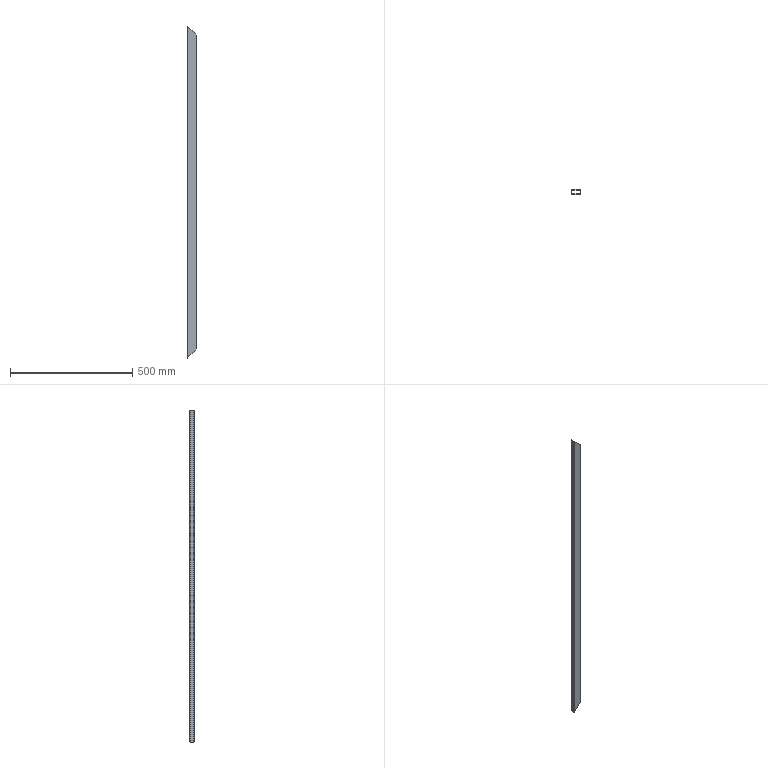Part | SolidWorks | features BaseBody 1 | 1 solid | 18 faces | box 40 x 20 x 1360 mm | volume 286615 mm3 | plane 10 | cylinder 8 | commonest cylinder face diameters 2 x4 6 x4
STEP:
#1=CARTESIAN_POINT('',(17.,-10.,643.));
#2=VERTEX_POINT('',#1);
#3=CARTESIAN_POINT('',(17.,-10.,-643.));
#4=VERTEX_POINT('',#3);
#5=CARTESIAN_POINT('',(17.,-10.,680.));
#6=DIRECTION('',(0.,0.,-1.));
#7=VECTOR('',#6,1000.);
#8=LINE('',#5,#7);
#9=EDGE_CURVE('',#2,#4,#8,.T.);
#10=ORIENTED_EDGE('',*,*,#9,.F.);
#11=CARTESIAN_POINT('',(-17.,-10.,677.));
#12=VERTEX_POINT('',#11);
#13=CARTESIAN_POINT('',(-20.,-10.,680.));
#14=DIRECTION('',(0.7071,0.,-0.7071));
#15=VECTOR('',#14,1000.);
#16=LINE('',#13,#15);
#17=EDGE_CURVE('',#12,#2,#16,.T.);
#18=ORIENTED_EDGE('',*,*,#17,.F.);
#19=CARTESIAN_POINT('',(-17.,-10.,-677.));
#20=VERTEX_POINT('',#19);
#21=CARTESIAN_POINT('',(-17.,-10.,680.));
#22=DIRECTION('',(0.,0.,-1.));
#23=VECTOR('',#22,1000.);
#24=LINE('',#21,#23);
#25=EDGE_CURVE('',#12,#20,#24,.T.);
#26=ORIENTED_EDGE('',*,*,#25,.T.);
#27=CARTESIAN_POINT('',(-20.,-10.,-680.));
#28=DIRECTION('',(-0.7071,0.,-0.7071));
#29=VECTOR('',#28,1000.);
#30=LINE('',#27,#29);
#31=EDGE_CURVE('',#4,#20,#30,.T.);
#32=ORIENTED_EDGE('',*,*,#31,.F.);
#33=EDGE_LOOP('',(#10,#18,#26,#32));
#34=FACE_OUTER_BOUND('',#33,.T.);
#35=CARTESIAN_POINT('',(-17.,-10.,680.));
#36=DIRECTION('',(0.,1.,0.));
#37=DIRECTION('',(1.,0.,0.));
#38=AXIS2_PLACEMENT_3D('',#35,#36,#37);
#39=PLANE('',#38);
#40=ADVANCED_FACE('',(#34),#39,.F.);
#41=ORIENTED_EDGE('',*,*,#25,.F.);
#42=CARTESIAN_POINT('',(-20.,-7.,680.));
#43=VERTEX_POINT('',#42);
#44=CARTESIAN_POINT('',(-17.,-10.,677.));
#45=CARTESIAN_POINT('',(-18.757,-10.,678.757));
#46=CARTESIAN_POINT('',(-20.,-8.757,680.));
#47=CARTESIAN_POINT('',(-20.,-7.,680.));
#48=(BOUNDED_CURVE()B_SPLINE_CURVE(3,(#44,#45,#46,#47),.UNSPECIFIED.,.F.,.T.)B_SPLINE_CURVE_WITH_KNOTS((4,4),(1.571,3.142),.UNSPECIFIED.)CURVE()GEOMETRIC_REPRESENTATION_ITEM()RATIONAL_B_SPLINE_CURVE((1.,0.8047,0.8047,1.))REPRESENTATION_ITEM(''));
#49=EDGE_CURVE('',#12,#43,#48,.T.);
#50=ORIENTED_EDGE('',*,*,#49,.T.);
#51=CARTESIAN_POINT('',(-20.,-7.,-680.));
#52=VERTEX_POINT('',#51);
#53=CARTESIAN_POINT('',(-20.,-7.,680.));
#54=DIRECTION('',(0.,0.,-1.));
#55=VECTOR('',#54,1000.);
#56=LINE('',#53,#55);
#57=EDGE_CURVE('',#43,#52,#56,.T.);
#58=ORIENTED_EDGE('',*,*,#57,.T.);
#59=CARTESIAN_POINT('',(-20.,-7.,-680.));
#60=CARTESIAN_POINT('',(-20.,-8.757,-680.));
#61=CARTESIAN_POINT('',(-18.757,-10.,-678.757));
#62=CARTESIAN_POINT('',(-17.,-10.,-677.));
#63=(BOUNDED_CURVE()B_SPLINE_CURVE(3,(#59,#60,#61,#62),.UNSPECIFIED.,.F.,.T.)B_SPLINE_CURVE_WITH_KNOTS((4,4),(0.,1.571),.UNSPECIFIED.)CURVE()GEOMETRIC_REPRESENTATION_ITEM()RATIONAL_B_SPLINE_CURVE((1.,0.8047,0.8047,1.))REPRESENTATION_ITEM(''));
#64=EDGE_CURVE('',#52,#20,#63,.T.);
#65=ORIENTED_EDGE('',*,*,#64,.T.);
#66=EDGE_LOOP('',(#41,#50,#58,#65));
#67=FACE_OUTER_BOUND('',#66,.T.);
#68=CARTESIAN_POINT('',(-17.,-7.,680.));
#69=DIRECTION('',(0.,0.,-1.));
#70=DIRECTION('',(-1.,0.,0.));
#71=AXIS2_PLACEMENT_3D('',#68,#69,#70);
#72=CYLINDRICAL_SURFACE('',#71,3.);
#73=ADVANCED_FACE('',(#67),#72,.T.);
#74=CARTESIAN_POINT('',(-20.,7.,-680.));
#75=VERTEX_POINT('',#74);
#76=CARTESIAN_POINT('',(-20.,7.,-680.));
#77=DIRECTION('',(0.,-1.,0.));
#78=VECTOR('',#77,1000.);
#79=LINE('',#76,#78);
#80=EDGE_CURVE('',#75,#52,#79,.T.);
#81=ORIENTED_EDGE('',*,*,#80,.T.);
#82=ORIENTED_EDGE('',*,*,#57,.F.);
#83=CARTESIAN_POINT('',(-20.,7.,680.));
#84=VERTEX_POINT('',#83);
#85=CARTESIAN_POINT('',(-20.,7.,680.));
#86=DIRECTION('',(0.,-1.,0.));
#87=VECTOR('',#86,1000.);
#88=LINE('',#85,#87);
#89=EDGE_CURVE('',#84,#43,#88,.T.);
#90=ORIENTED_EDGE('',*,*,#89,.F.);
#91=CARTESIAN_POINT('',(-20.,7.,680.));
#92=DIRECTION('',(0.,0.,-1.));
#93=VECTOR('',#92,1000.);
#94=LINE('',#91,#93);
#95=EDGE_CURVE('',#84,#75,#94,.T.);
#96=ORIENTED_EDGE('',*,*,#95,.T.);
#97=EDGE_LOOP('',(#81,#82,#90,#96));
#98=FACE_OUTER_BOUND('',#97,.T.);
#99=CARTESIAN_POINT('',(-20.,7.,680.));
#100=DIRECTION('',(1.,0.,0.));
#101=DIRECTION('',(0.,1.,0.));
#102=AXIS2_PLACEMENT_3D('',#99,#100,#101);
#103=PLANE('',#102);
#104=ADVANCED_FACE('',(#98),#103,.F.);
#105=ORIENTED_EDGE('',*,*,#95,.F.);
#106=CARTESIAN_POINT('',(-17.,10.,677.));
#107=VERTEX_POINT('',#106);
#108=CARTESIAN_POINT('',(-20.,7.,680.));
#109=CARTESIAN_POINT('',(-20.,8.757,680.));
#110=CARTESIAN_POINT('',(-18.757,10.,678.757));
#111=CARTESIAN_POINT('',(-17.,10.,677.));
#112=(BOUNDED_CURVE()B_SPLINE_CURVE(3,(#108,#109,#110,#111),.UNSPECIFIED.,.F.,.T.)B_SPLINE_CURVE_WITH_KNOTS((4,4),(3.142,4.712),.UNSPECIFIED.)CURVE()GEOMETRIC_REPRESENTATION_ITEM()RATIONAL_B_SPLINE_CURVE((1.,0.8047,0.8047,1.))REPRESENTATION_ITEM(''));
#113=EDGE_CURVE('',#84,#107,#112,.T.);
#114=ORIENTED_EDGE('',*,*,#113,.T.);
#115=CARTESIAN_POINT('',(-17.,10.,-677.));
#116=VERTEX_POINT('',#115);
#117=CARTESIAN_POINT('',(-17.,10.,680.));
#118=DIRECTION('',(0.,0.,-1.));
#119=VECTOR('',#118,1000.);
#120=LINE('',#117,#119);
#121=EDGE_CURVE('',#107,#116,#120,.T.);
#122=ORIENTED_EDGE('',*,*,#121,.T.);
#123=CARTESIAN_POINT('',(-17.,10.,-677.));
#124=CARTESIAN_POINT('',(-18.757,10.,-678.757));
#125=CARTESIAN_POINT('',(-20.,8.757,-680.));
#126=CARTESIAN_POINT('',(-20.,7.,-680.));
#127=(BOUNDED_CURVE()B_SPLINE_CURVE(3,(#123,#124,#125,#126),.UNSPECIFIED.,.F.,.F.)B_SPLINE_CURVE_WITH_KNOTS((4,4),(4.712,6.283),.UNSPECIFIED.)CURVE()GEOMETRIC_REPRESENTATION_ITEM()RATIONAL_B_SPLINE_CURVE((1.,0.8047,0.8047,1.))REPRESENTATION_ITEM(''));
#128=EDGE_CURVE('',#116,#75,#127,.T.);
#129=ORIENTED_EDGE('',*,*,#128,.T.);
#130=EDGE_LOOP('',(#105,#114,#122,#129));
#131=FACE_OUTER_BOUND('',#130,.T.);
#132=CARTESIAN_POINT('',(-17.,7.,680.));
#133=DIRECTION('',(0.,0.,-1.));
#134=DIRECTION('',(-1.,0.,0.));
#135=AXIS2_PLACEMENT_3D('',#132,#133,#134);
#136=CYLINDRICAL_SURFACE('',#135,3.);
#137=ADVANCED_FACE('',(#131),#136,.T.);
#138=ORIENTED_EDGE('',*,*,#121,.F.);
#139=CARTESIAN_POINT('',(17.,10.,643.));
#140=VERTEX_POINT('',#139);
#141=CARTESIAN_POINT('',(-20.,10.,680.));
#142=DIRECTION('',(0.7071,0.,-0.7071));
#143=VECTOR('',#142,1000.);
#144=LINE('',#141,#143);
#145=EDGE_CURVE('',#107,#140,#144,.T.);
#146=ORIENTED_EDGE('',*,*,#145,.T.);
#147=CARTESIAN_POINT('',(17.,10.,-643.));
#148=VERTEX_POINT('',#147);
#149=CARTESIAN_POINT('',(17.,10.,680.));
#150=DIRECTION('',(0.,0.,-1.));
#151=VECTOR('',#150,1000.);
#152=LINE('',#149,#151);
#153=EDGE_CURVE('',#140,#148,#152,.T.);
#154=ORIENTED_EDGE('',*,*,#153,.T.);
#155=CARTESIAN_POINT('',(-20.,10.,-680.));
#156=DIRECTION('',(-0.7071,0.,-0.7071));
#157=VECTOR('',#156,1000.);
#158=LINE('',#155,#157);
#159=EDGE_CURVE('',#148,#116,#158,.T.);
#160=ORIENTED_EDGE('',*,*,#159,.T.);
#161=EDGE_LOOP('',(#138,#146,#154,#160));
#162=FACE_OUTER_BOUND('',#161,.T.);
#163=CARTESIAN_POINT('',(-17.,10.,680.));
#164=DIRECTION('',(0.,-1.,0.));
#165=DIRECTION('',(0.,0.,-1.));
#166=AXIS2_PLACEMENT_3D('',#163,#164,#165);
#167=PLANE('',#166);
#168=ADVANCED_FACE('',(#162),#167,.F.);
#169=ORIENTED_EDGE('',*,*,#153,.F.);
#170=CARTESIAN_POINT('',(20.,7.,640.));
#171=VERTEX_POINT('',#170);
#172=CARTESIAN_POINT('',(17.,10.,643.));
#173=CARTESIAN_POINT('',(18.757,10.,641.243));
#174=CARTESIAN_POINT('',(20.,8.757,640.));
#175=CARTESIAN_POINT('',(20.,7.,640.));
#176=(BOUNDED_CURVE()B_SPLINE_CURVE(3,(#172,#173,#174,#175),.UNSPECIFIED.,.F.,.T.)B_SPLINE_CURVE_WITH_KNOTS((4,4),(4.712,6.283),.UNSPECIFIED.)CURVE()GEOMETRIC_REPRESENTATION_ITEM()RATIONAL_B_SPLINE_CURVE((1.,0.8047,0.8047,1.))REPRESENTATION_ITEM(''));
#177=EDGE_CURVE('',#140,#171,#176,.T.);
#178=ORIENTED_EDGE('',*,*,#177,.T.);
#179=CARTESIAN_POINT('',(20.,7.,-640.));
#180=VERTEX_POINT('',#179);
#181=CARTESIAN_POINT('',(20.,7.,680.));
#182=DIRECTION('',(0.,0.,-1.));
#183=VECTOR('',#182,1000.);
#184=LINE('',#181,#183);
#185=EDGE_CURVE('',#171,#180,#184,.T.);
#186=ORIENTED_EDGE('',*,*,#185,.T.);
#187=CARTESIAN_POINT('',(20.,7.,-640.));
#188=CARTESIAN_POINT('',(20.,8.757,-640.));
#189=CARTESIAN_POINT('',(18.757,10.,-641.243));
#190=CARTESIAN_POINT('',(17.,10.,-643.));
#191=(BOUNDED_CURVE()B_SPLINE_CURVE(3,(#187,#188,#189,#190),.UNSPECIFIED.,.F.,.T.)B_SPLINE_CURVE_WITH_KNOTS((4,4),(3.142,4.712),.UNSPECIFIED.)CURVE()GEOMETRIC_REPRESENTATION_ITEM()RATIONAL_B_SPLINE_CURVE((1.,0.8047,0.8047,1.))REPRESENTATION_ITEM(''));
#192=EDGE_CURVE('',#180,#148,#191,.T.);
#193=ORIENTED_EDGE('',*,*,#192,.T.);
#194=EDGE_LOOP('',(#169,#178,#186,#193));
#195=FACE_OUTER_BOUND('',#194,.T.);
#196=CARTESIAN_POINT('',(17.,7.,680.));
#197=DIRECTION('',(0.,0.,-1.));
#198=DIRECTION('',(-1.,0.,0.));
#199=AXIS2_PLACEMENT_3D('',#196,#197,#198);
#200=CYLINDRICAL_SURFACE('',#199,3.);
#201=ADVANCED_FACE('',(#195),#200,.T.);
#202=ORIENTED_EDGE('',*,*,#185,.F.);
#203=CARTESIAN_POINT('',(20.,-7.,640.));
#204=VERTEX_POINT('',#203);
#205=CARTESIAN_POINT('',(20.,10.,640.));
#206=DIRECTION('',(0.,-1.,0.));
#207=VECTOR('',#206,1000.);
#208=LINE('',#205,#207);
#209=EDGE_CURVE('',#171,#204,#208,.T.);
#210=ORIENTED_EDGE('',*,*,#209,.T.);
#211=CARTESIAN_POINT('',(20.,-7.,-640.));
#212=VERTEX_POINT('',#211);
#213=CARTESIAN_POINT('',(20.,-7.,680.));
#214=DIRECTION('',(0.,0.,-1.));
#215=VECTOR('',#214,1000.);
#216=LINE('',#213,#215);
#217=EDGE_CURVE('',#204,#212,#216,.T.);
#218=ORIENTED_EDGE('',*,*,#217,.T.);
#219=CARTESIAN_POINT('',(20.,10.,-640.));
#220=DIRECTION('',(0.,-1.,0.));
#221=VECTOR('',#220,1000.);
#222=LINE('',#219,#221);
#223=EDGE_CURVE('',#180,#212,#222,.T.);
#224=ORIENTED_EDGE('',*,*,#223,.F.);
#225=EDGE_LOOP('',(#202,#210,#218,#224));
#226=FACE_OUTER_BOUND('',#225,.T.);
#227=CARTESIAN_POINT('',(20.,7.,680.));
#228=DIRECTION('',(-1.,0.,0.));
#229=DIRECTION('',(0.,0.,1.));
#230=AXIS2_PLACEMENT_3D('',#227,#228,#229);
#231=PLANE('',#230);
#232=ADVANCED_FACE('',(#226),#231,.F.);
#233=ORIENTED_EDGE('',*,*,#217,.F.);
#234=CARTESIAN_POINT('',(20.,-7.,640.));
#235=CARTESIAN_POINT('',(20.,-8.757,640.));
#236=CARTESIAN_POINT('',(18.757,-10.,641.243));
#237=CARTESIAN_POINT('',(17.,-10.,643.));
#238=(BOUNDED_CURVE()B_SPLINE_CURVE(3,(#234,#235,#236,#237),.UNSPECIFIED.,.F.,.T.)B_SPLINE_CURVE_WITH_KNOTS((4,4),(0.,1.571),.UNSPECIFIED.)CURVE()GEOMETRIC_REPRESENTATION_ITEM()RATIONAL_B_SPLINE_CURVE((1.,0.8047,0.8047,1.))REPRESENTATION_ITEM(''));
#239=EDGE_CURVE('',#204,#2,#238,.T.);
#240=ORIENTED_EDGE('',*,*,#239,.T.);
#241=ORIENTED_EDGE('',*,*,#9,.T.);
#242=CARTESIAN_POINT('',(17.,-10.,-643.));
#243=CARTESIAN_POINT('',(18.757,-10.,-641.243));
#244=CARTESIAN_POINT('',(20.,-8.757,-640.));
#245=CARTESIAN_POINT('',(20.,-7.,-640.));
#246=(BOUNDED_CURVE()B_SPLINE_CURVE(3,(#242,#243,#244,#245),.UNSPECIFIED.,.F.,.T.)B_SPLINE_CURVE_WITH_KNOTS((4,4),(1.571,3.142),.UNSPECIFIED.)CURVE()GEOMETRIC_REPRESENTATION_ITEM()RATIONAL_B_SPLINE_CURVE((1.,0.8047,0.8047,1.))REPRESENTATION_ITEM(''));
#247=EDGE_CURVE('',#4,#212,#246,.T.);
#248=ORIENTED_EDGE('',*,*,#247,.T.);
#249=EDGE_LOOP('',(#233,#240,#241,#248));
#250=FACE_OUTER_BOUND('',#249,.T.);
#251=CARTESIAN_POINT('',(17.,-7.,680.));
#252=DIRECTION('',(0.,0.,-1.));
#253=DIRECTION('',(-1.,0.,0.));
#254=AXIS2_PLACEMENT_3D('',#251,#252,#253);
#255=CYLINDRICAL_SURFACE('',#254,3.);
#256=ADVANCED_FACE('',(#250),#255,.T.);
#257=CARTESIAN_POINT('',(17.,8.,643.));
#258=VERTEX_POINT('',#257);
#259=CARTESIAN_POINT('',(18.,7.,642.));
#260=VERTEX_POINT('',#259);
#261=CARTESIAN_POINT('',(17.,8.,643.));
#262=CARTESIAN_POINT('',(17.586,8.,642.414));
#263=CARTESIAN_POINT('',(18.,7.586,642.));
#264=CARTESIAN_POINT('',(18.,7.,642.));
#265=(BOUNDED_CURVE()B_SPLINE_CURVE(3,(#261,#262,#263,#264),.UNSPECIFIED.,.F.,.F.)B_SPLINE_CURVE_WITH_KNOTS((4,4),(4.712,6.283),.UNSPECIFIED.)CURVE()GEOMETRIC_REPRESENTATION_ITEM()RATIONAL_B_SPLINE_CURVE((1.,0.8047,0.8047,1.))REPRESENTATION_ITEM(''));
#266=EDGE_CURVE('',#258,#260,#265,.T.);
#267=ORIENTED_EDGE('',*,*,#266,.T.);
#268=CARTESIAN_POINT('',(18.,-7.,642.));
#269=VERTEX_POINT('',#268);
#270=CARTESIAN_POINT('',(18.,7.,642.));
#271=DIRECTION('',(0.,-1.,0.));
#272=VECTOR('',#271,1000.);
#273=LINE('',#270,#272);
#274=EDGE_CURVE('',#260,#269,#273,.T.);
#275=ORIENTED_EDGE('',*,*,#274,.T.);
#276=CARTESIAN_POINT('',(17.,-8.,643.));
#277=VERTEX_POINT('',#276);
#278=CARTESIAN_POINT('',(18.,-7.,642.));
#279=CARTESIAN_POINT('',(18.,-7.586,642.));
#280=CARTESIAN_POINT('',(17.586,-8.,642.414));
#281=CARTESIAN_POINT('',(17.,-8.,643.));
#282=(BOUNDED_CURVE()B_SPLINE_CURVE(3,(#278,#279,#280,#281),.UNSPECIFIED.,.F.,.T.)B_SPLINE_CURVE_WITH_KNOTS((4,4),(0.,1.571),.UNSPECIFIED.)CURVE()GEOMETRIC_REPRESENTATION_ITEM()RATIONAL_B_SPLINE_CURVE((1.,0.8047,0.8047,1.))REPRESENTATION_ITEM(''));
#283=EDGE_CURVE('',#269,#277,#282,.T.);
#284=ORIENTED_EDGE('',*,*,#283,.T.);
#285=CARTESIAN_POINT('',(-17.,-8.,677.));
#286=VERTEX_POINT('',#285);
#287=CARTESIAN_POINT('',(-18.5,-8.,678.5));
#288=DIRECTION('',(-0.7071,0.,0.7071));
#289=VECTOR('',#288,1000.);
#290=LINE('',#287,#289);
#291=EDGE_CURVE('',#277,#286,#290,.T.);
#292=ORIENTED_EDGE('',*,*,#291,.T.);
#293=CARTESIAN_POINT('',(-18.,-7.,678.));
#294=VERTEX_POINT('',#293);
#295=CARTESIAN_POINT('',(-17.,-8.,677.));
#296=CARTESIAN_POINT('',(-17.586,-8.,677.586));
#297=CARTESIAN_POINT('',(-18.,-7.586,678.));
#298=CARTESIAN_POINT('',(-18.,-7.,678.));
#299=(BOUNDED_CURVE()B_SPLINE_CURVE(3,(#295,#296,#297,#298),.UNSPECIFIED.,.F.,.T.)B_SPLINE_CURVE_WITH_KNOTS((4,4),(1.571,3.142),.UNSPECIFIED.)CURVE()GEOMETRIC_REPRESENTATION_ITEM()RATIONAL_B_SPLINE_CURVE((1.,0.8047,0.8047,1.))REPRESENTATION_ITEM(''));
#300=EDGE_CURVE('',#286,#294,#299,.T.);
#301=ORIENTED_EDGE('',*,*,#300,.T.);
#302=CARTESIAN_POINT('',(-18.,7.,678.));
#303=VERTEX_POINT('',#302);
#304=CARTESIAN_POINT('',(-18.,7.,678.));
#305=DIRECTION('',(0.,1.,0.));
#306=VECTOR('',#305,1000.);
#307=LINE('',#304,#306);
#308=EDGE_CURVE('',#294,#303,#307,.T.);
#309=ORIENTED_EDGE('',*,*,#308,.T.);
#310=CARTESIAN_POINT('',(-17.,8.,677.));
#311=VERTEX_POINT('',#310);
#312=CARTESIAN_POINT('',(-18.,7.,678.));
#313=CARTESIAN_POINT('',(-18.,7.586,678.));
#314=CARTESIAN_POINT('',(-17.586,8.,677.586));
#315=CARTESIAN_POINT('',(-17.,8.,677.));
#316=(BOUNDED_CURVE()B_SPLINE_CURVE(3,(#312,#313,#314,#315),.UNSPECIFIED.,.F.,.T.)B_SPLINE_CURVE_WITH_KNOTS((4,4),(3.142,4.712),.UNSPECIFIED.)CURVE()GEOMETRIC_REPRESENTATION_ITEM()RATIONAL_B_SPLINE_CURVE((1.,0.8047,0.8047,1.))REPRESENTATION_ITEM(''));
#317=EDGE_CURVE('',#303,#311,#316,.T.);
#318=ORIENTED_EDGE('',*,*,#317,.T.);
#319=CARTESIAN_POINT('',(-18.5,8.,678.5));
#320=DIRECTION('',(0.7071,0.,-0.7071));
#321=VECTOR('',#320,1000.);
#322=LINE('',#319,#321);
#323=EDGE_CURVE('',#311,#258,#322,.T.);
#324=ORIENTED_EDGE('',*,*,#323,.T.);
#325=EDGE_LOOP('',(#267,#275,#284,#292,#301,#309,#318,#324));
#326=FACE_BOUND('',#325,.T.);
#327=ORIENTED_EDGE('',*,*,#209,.F.);
#328=ORIENTED_EDGE('',*,*,#177,.F.);
#329=ORIENTED_EDGE('',*,*,#145,.F.);
#330=ORIENTED_EDGE('',*,*,#113,.F.);
#331=ORIENTED_EDGE('',*,*,#89,.T.);
#332=ORIENTED_EDGE('',*,*,#49,.F.);
#333=ORIENTED_EDGE('',*,*,#17,.T.);
#334=ORIENTED_EDGE('',*,*,#239,.F.);
#335=EDGE_LOOP('',(#327,#328,#329,#330,#331,#332,#333,#334));
#336=FACE_OUTER_BOUND('',#335,.T.);
#337=CARTESIAN_POINT('',(-20.,10.,680.));
#338=DIRECTION('',(-0.7071,0.,-0.7071));
#339=DIRECTION('',(-0.7071,0.,0.7071));
#340=AXIS2_PLACEMENT_3D('',#337,#338,#339);
#341=PLANE('',#340);
#342=ADVANCED_FACE('',(#326,#336),#341,.F.);
#343=CARTESIAN_POINT('',(18.,7.,-642.));
#344=VERTEX_POINT('',#343);
#345=CARTESIAN_POINT('',(17.,8.,-643.));
#346=VERTEX_POINT('',#345);
#347=CARTESIAN_POINT('',(18.,7.,-642.));
#348=CARTESIAN_POINT('',(18.,7.586,-642.));
#349=CARTESIAN_POINT('',(17.586,8.,-642.414));
#350=CARTESIAN_POINT('',(17.,8.,-643.));
#351=(BOUNDED_CURVE()B_SPLINE_CURVE(3,(#347,#348,#349,#350),.UNSPECIFIED.,.F.,.T.)B_SPLINE_CURVE_WITH_KNOTS((4,4),(3.142,4.712),.UNSPECIFIED.)CURVE()GEOMETRIC_REPRESENTATION_ITEM()RATIONAL_B_SPLINE_CURVE((1.,0.8047,0.8047,1.))REPRESENTATION_ITEM(''));
#352=EDGE_CURVE('',#344,#346,#351,.T.);
#353=ORIENTED_EDGE('',*,*,#352,.T.);
#354=CARTESIAN_POINT('',(-17.,8.,-677.));
#355=VERTEX_POINT('',#354);
#356=CARTESIAN_POINT('',(661.5,8.,1.5));
#357=DIRECTION('',(-0.7071,0.,-0.7071));
#358=VECTOR('',#357,1000.);
#359=LINE('',#356,#358);
#360=EDGE_CURVE('',#346,#355,#359,.T.);
#361=ORIENTED_EDGE('',*,*,#360,.T.);
#362=CARTESIAN_POINT('',(-18.,7.,-678.));
#363=VERTEX_POINT('',#362);
#364=CARTESIAN_POINT('',(-17.,8.,-677.));
#365=CARTESIAN_POINT('',(-17.586,8.,-677.586));
#366=CARTESIAN_POINT('',(-18.,7.586,-678.));
#367=CARTESIAN_POINT('',(-18.,7.,-678.));
#368=(BOUNDED_CURVE()B_SPLINE_CURVE(3,(#364,#365,#366,#367),.UNSPECIFIED.,.F.,.T.)B_SPLINE_CURVE_WITH_KNOTS((4,4),(4.712,6.283),.UNSPECIFIED.)CURVE()GEOMETRIC_REPRESENTATION_ITEM()RATIONAL_B_SPLINE_CURVE((1.,0.8047,0.8047,1.))REPRESENTATION_ITEM(''));
#369=EDGE_CURVE('',#355,#363,#368,.T.);
#370=ORIENTED_EDGE('',*,*,#369,.T.);
#371=CARTESIAN_POINT('',(-18.,-7.,-678.));
#372=VERTEX_POINT('',#371);
#373=CARTESIAN_POINT('',(-18.,7.,-678.));
#374=DIRECTION('',(0.,-1.,0.));
#375=VECTOR('',#374,1000.);
#376=LINE('',#373,#375);
#377=EDGE_CURVE('',#363,#372,#376,.T.);
#378=ORIENTED_EDGE('',*,*,#377,.T.);
#379=CARTESIAN_POINT('',(-17.,-8.,-677.));
#380=VERTEX_POINT('',#379);
#381=CARTESIAN_POINT('',(-18.,-7.,-678.));
#382=CARTESIAN_POINT('',(-18.,-7.586,-678.));
#383=CARTESIAN_POINT('',(-17.586,-8.,-677.586));
#384=CARTESIAN_POINT('',(-17.,-8.,-677.));
#385=(BOUNDED_CURVE()B_SPLINE_CURVE(3,(#381,#382,#383,#384),.UNSPECIFIED.,.F.,.T.)B_SPLINE_CURVE_WITH_KNOTS((4,4),(0.,1.571),.UNSPECIFIED.)CURVE()GEOMETRIC_REPRESENTATION_ITEM()RATIONAL_B_SPLINE_CURVE((1.,0.8047,0.8047,1.))REPRESENTATION_ITEM(''));
#386=EDGE_CURVE('',#372,#380,#385,.T.);
#387=ORIENTED_EDGE('',*,*,#386,.T.);
#388=CARTESIAN_POINT('',(17.,-8.,-643.));
#389=VERTEX_POINT('',#388);
#390=CARTESIAN_POINT('',(661.5,-8.,1.5));
#391=DIRECTION('',(0.7071,0.,0.7071));
#392=VECTOR('',#391,1000.);
#393=LINE('',#390,#392);
#394=EDGE_CURVE('',#380,#389,#393,.T.);
#395=ORIENTED_EDGE('',*,*,#394,.T.);
#396=CARTESIAN_POINT('',(18.,-7.,-642.));
#397=VERTEX_POINT('',#396);
#398=CARTESIAN_POINT('',(17.,-8.,-643.));
#399=CARTESIAN_POINT('',(17.586,-8.,-642.414));
#400=CARTESIAN_POINT('',(18.,-7.586,-642.));
#401=CARTESIAN_POINT('',(18.,-7.,-642.));
#402=(BOUNDED_CURVE()B_SPLINE_CURVE(3,(#398,#399,#400,#401),.UNSPECIFIED.,.F.,.T.)B_SPLINE_CURVE_WITH_KNOTS((4,4),(1.571,3.142),.UNSPECIFIED.)CURVE()GEOMETRIC_REPRESENTATION_ITEM()RATIONAL_B_SPLINE_CURVE((1.,0.8047,0.8047,1.))REPRESENTATION_ITEM(''));
#403=EDGE_CURVE('',#389,#397,#402,.T.);
#404=ORIENTED_EDGE('',*,*,#403,.T.);
#405=CARTESIAN_POINT('',(18.,7.,-642.));
#406=DIRECTION('',(0.,1.,0.));
#407=VECTOR('',#406,1000.);
#408=LINE('',#405,#407);
#409=EDGE_CURVE('',#397,#344,#408,.T.);
#410=ORIENTED_EDGE('',*,*,#409,.T.);
#411=EDGE_LOOP('',(#353,#361,#370,#378,#387,#395,#404,#410));
#412=FACE_BOUND('',#411,.T.);
#413=ORIENTED_EDGE('',*,*,#31,.T.);
#414=ORIENTED_EDGE('',*,*,#64,.F.);
#415=ORIENTED_EDGE('',*,*,#80,.F.);
#416=ORIENTED_EDGE('',*,*,#128,.F.);
#417=ORIENTED_EDGE('',*,*,#159,.F.);
#418=ORIENTED_EDGE('',*,*,#192,.F.);
#419=ORIENTED_EDGE('',*,*,#223,.T.);
#420=ORIENTED_EDGE('',*,*,#247,.F.);
#421=EDGE_LOOP('',(#413,#414,#415,#416,#417,#418,#419,#420));
#422=FACE_OUTER_BOUND('',#421,.T.);
#423=CARTESIAN_POINT('',(-20.,10.,-680.));
#424=DIRECTION('',(-0.7071,0.,0.7071));
#425=DIRECTION('',(0.,1.,0.));
#426=AXIS2_PLACEMENT_3D('',#423,#424,#425);
#427=PLANE('',#426);
#428=ADVANCED_FACE('',(#412,#422),#427,.F.);
#429=ORIENTED_EDGE('',*,*,#266,.F.);
#430=CARTESIAN_POINT('',(17.,8.,680.));
#431=DIRECTION('',(0.,0.,-1.));
#432=VECTOR('',#431,1000.);
#433=LINE('',#430,#432);
#434=EDGE_CURVE('',#258,#346,#433,.T.);
#435=ORIENTED_EDGE('',*,*,#434,.T.);
#436=ORIENTED_EDGE('',*,*,#352,.F.);
#437=CARTESIAN_POINT('',(18.,7.,680.));
#438=DIRECTION('',(0.,0.,-1.));
#439=VECTOR('',#438,1000.);
#440=LINE('',#437,#439);
#441=EDGE_CURVE('',#260,#344,#440,.T.);
#442=ORIENTED_EDGE('',*,*,#441,.F.);
#443=EDGE_LOOP('',(#429,#435,#436,#442));
#444=FACE_OUTER_BOUND('',#443,.T.);
#445=CARTESIAN_POINT('',(17.,7.,680.));
#446=DIRECTION('',(0.,0.,-1.));
#447=DIRECTION('',(-1.,0.,0.));
#448=AXIS2_PLACEMENT_3D('',#445,#446,#447);
#449=CYLINDRICAL_SURFACE('',#448,1.);
#450=ADVANCED_FACE('',(#444),#449,.F.);
#451=ORIENTED_EDGE('',*,*,#323,.F.);
#452=CARTESIAN_POINT('',(-17.,8.,680.));
#453=DIRECTION('',(0.,0.,-1.));
#454=VECTOR('',#453,1000.);
#455=LINE('',#452,#454);
#456=EDGE_CURVE('',#311,#355,#455,.T.);
#457=ORIENTED_EDGE('',*,*,#456,.T.);
#458=ORIENTED_EDGE('',*,*,#360,.F.);
#459=ORIENTED_EDGE('',*,*,#434,.F.);
#460=EDGE_LOOP('',(#451,#457,#458,#459));
#461=FACE_OUTER_BOUND('',#460,.T.);
#462=CARTESIAN_POINT('',(-17.,8.,680.));
#463=DIRECTION('',(0.,-1.,0.));
#464=DIRECTION('',(0.,0.,-1.));
#465=AXIS2_PLACEMENT_3D('',#462,#463,#464);
#466=PLANE('',#465);
#467=ADVANCED_FACE('',(#461),#466,.T.);
#468=ORIENTED_EDGE('',*,*,#317,.F.);
#469=CARTESIAN_POINT('',(-18.,7.,680.));
#470=DIRECTION('',(0.,0.,-1.));
#471=VECTOR('',#470,1000.);
#472=LINE('',#469,#471);
#473=EDGE_CURVE('',#303,#363,#472,.T.);
#474=ORIENTED_EDGE('',*,*,#473,.T.);
#475=ORIENTED_EDGE('',*,*,#369,.F.);
#476=ORIENTED_EDGE('',*,*,#456,.F.);
#477=EDGE_LOOP('',(#468,#474,#475,#476));
#478=FACE_OUTER_BOUND('',#477,.T.);
#479=CARTESIAN_POINT('',(-17.,7.,680.));
#480=DIRECTION('',(0.,0.,-1.));
#481=DIRECTION('',(-1.,0.,0.));
#482=AXIS2_PLACEMENT_3D('',#479,#480,#481);
#483=CYLINDRICAL_SURFACE('',#482,1.);
#484=ADVANCED_FACE('',(#478),#483,.F.);
#485=ORIENTED_EDGE('',*,*,#308,.F.);
#486=CARTESIAN_POINT('',(-18.,-7.,680.));
#487=DIRECTION('',(0.,0.,-1.));
#488=VECTOR('',#487,1000.);
#489=LINE('',#486,#488);
#490=EDGE_CURVE('',#294,#372,#489,.T.);
#491=ORIENTED_EDGE('',*,*,#490,.T.);
#492=ORIENTED_EDGE('',*,*,#377,.F.);
#493=ORIENTED_EDGE('',*,*,#473,.F.);
#494=EDGE_LOOP('',(#485,#491,#492,#493));
#495=FACE_OUTER_BOUND('',#494,.T.);
#496=CARTESIAN_POINT('',(-18.,7.,680.));
#497=DIRECTION('',(1.,0.,0.));
#498=DIRECTION('',(0.,-1.,0.));
#499=AXIS2_PLACEMENT_3D('',#496,#497,#498);
#500=PLANE('',#499);
#501=ADVANCED_FACE('',(#495),#500,.T.);
#502=ORIENTED_EDGE('',*,*,#300,.F.);
#503=CARTESIAN_POINT('',(-17.,-8.,680.));
#504=DIRECTION('',(0.,0.,-1.));
#505=VECTOR('',#504,1000.);
#506=LINE('',#503,#505);
#507=EDGE_CURVE('',#286,#380,#506,.T.);
#508=ORIENTED_EDGE('',*,*,#507,.T.);
#509=ORIENTED_EDGE('',*,*,#386,.F.);
#510=ORIENTED_EDGE('',*,*,#490,.F.);
#511=EDGE_LOOP('',(#502,#508,#509,#510));
#512=FACE_OUTER_BOUND('',#511,.T.);
#513=CARTESIAN_POINT('',(-17.,-7.,680.));
#514=DIRECTION('',(0.,0.,-1.));
#515=DIRECTION('',(-1.,0.,0.));
#516=AXIS2_PLACEMENT_3D('',#513,#514,#515);
#517=CYLINDRICAL_SURFACE('',#516,1.);
#518=ADVANCED_FACE('',(#512),#517,.F.);
#519=ORIENTED_EDGE('',*,*,#291,.F.);
#520=CARTESIAN_POINT('',(17.,-8.,680.));
#521=DIRECTION('',(0.,0.,-1.));
#522=VECTOR('',#521,1000.);
#523=LINE('',#520,#522);
#524=EDGE_CURVE('',#277,#389,#523,.T.);
#525=ORIENTED_EDGE('',*,*,#524,.T.);
#526=ORIENTED_EDGE('',*,*,#394,.F.);
#527=ORIENTED_EDGE('',*,*,#507,.F.);
#528=EDGE_LOOP('',(#519,#525,#526,#527));
#529=FACE_OUTER_BOUND('',#528,.T.);
#530=CARTESIAN_POINT('',(-17.,-8.,680.));
#531=DIRECTION('',(0.,1.,0.));
#532=DIRECTION('',(1.,0.,0.));
#533=AXIS2_PLACEMENT_3D('',#530,#531,#532);
#534=PLANE('',#533);
#535=ADVANCED_FACE('',(#529),#534,.T.);
#536=ORIENTED_EDGE('',*,*,#283,.F.);
#537=CARTESIAN_POINT('',(18.,-7.,680.));
#538=DIRECTION('',(0.,0.,-1.));
#539=VECTOR('',#538,1000.);
#540=LINE('',#537,#539);
#541=EDGE_CURVE('',#269,#397,#540,.T.);
#542=ORIENTED_EDGE('',*,*,#541,.T.);
#543=ORIENTED_EDGE('',*,*,#403,.F.);
#544=ORIENTED_EDGE('',*,*,#524,.F.);
#545=EDGE_LOOP('',(#536,#542,#543,#544));
#546=FACE_OUTER_BOUND('',#545,.T.);
#547=CARTESIAN_POINT('',(17.,-7.,680.));
#548=DIRECTION('',(0.,0.,-1.));
#549=DIRECTION('',(-1.,0.,0.));
#550=AXIS2_PLACEMENT_3D('',#547,#548,#549);
#551=CYLINDRICAL_SURFACE('',#550,1.);
#552=ADVANCED_FACE('',(#546),#551,.F.);
#553=ORIENTED_EDGE('',*,*,#274,.F.);
#554=ORIENTED_EDGE('',*,*,#441,.T.);
#555=ORIENTED_EDGE('',*,*,#409,.F.);
#556=ORIENTED_EDGE('',*,*,#541,.F.);
#557=EDGE_LOOP('',(#553,#554,#555,#556));
#558=FACE_OUTER_BOUND('',#557,.T.);
#559=CARTESIAN_POINT('',(18.,7.,680.));
#560=DIRECTION('',(-1.,0.,0.));
#561=DIRECTION('',(0.,0.,1.));
#562=AXIS2_PLACEMENT_3D('',#559,#560,#561);
#563=PLANE('',#562);
#564=ADVANCED_FACE('',(#558),#563,.T.);
#565=CLOSED_SHELL('',(#40,#73,#104,#137,#168,#201,#232,#256,#342,#428,#450,#467,#484,#501,#518,#535,#552,#564));
#566=MANIFOLD_SOLID_BREP('',#565);
#567=CARTESIAN_POINT('',(0.,0.,0.));
#568=DIRECTION('',(0.,0.,1.));
#569=DIRECTION('',(1.,0.,0.));
#570=AXIS2_PLACEMENT_3D('',#567,#568,#569);
#571=(LENGTH_UNIT()NAMED_UNIT(*)SI_UNIT(.MILLI.,.METRE.));
#572=UNCERTAINTY_MEASURE_WITH_UNIT(LENGTH_MEASURE(0.00001),#571,'','');
#573=(NAMED_UNIT(*)PLANE_ANGLE_UNIT()SI_UNIT($,.RADIAN.));
#574=(NAMED_UNIT(*)SI_UNIT($,.STERADIAN.)SOLID_ANGLE_UNIT());
#575=(GEOMETRIC_REPRESENTATION_CONTEXT(3)GLOBAL_UNCERTAINTY_ASSIGNED_CONTEXT((#572))GLOBAL_UNIT_ASSIGNED_CONTEXT((#571,#573,#574))REPRESENTATION_CONTEXT('',''));
#576=ADVANCED_BREP_SHAPE_REPRESENTATION('',(#566,#570),#575);